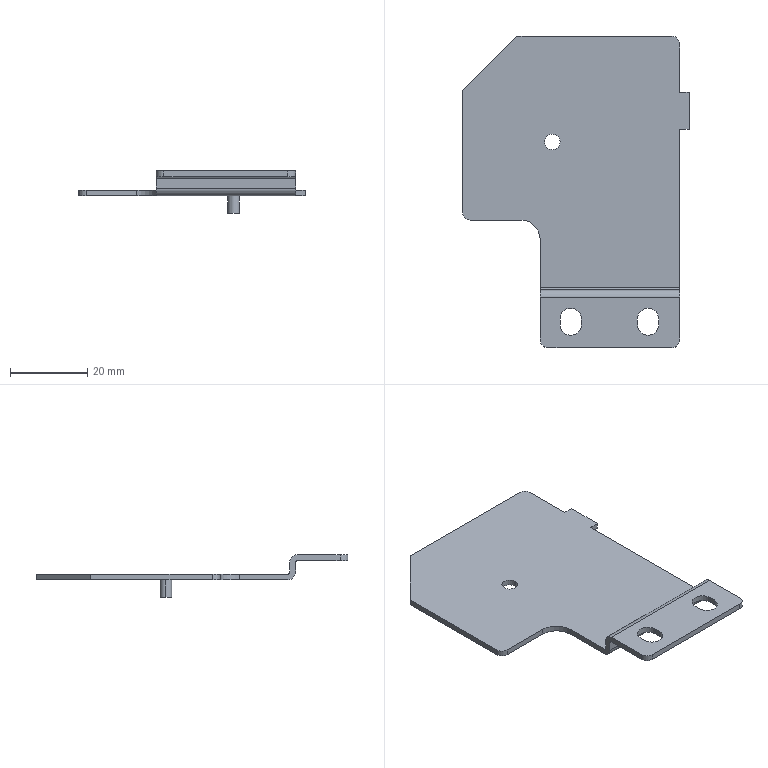Part | NX | features BREP 1 | 1 solid | 39 faces | box 58.5 x 80.5 x 11 mm | volume 5793 mm3 | plane 22 | cylinder 17 | commonest cylinder face diameters 4 x8 5.5 x4 1 x2 3 x2 10 x1
STEP:
#1=CARTESIAN_POINT('',(-6.875,12.95,1.));
#2=VERTEX_POINT('',#1);
#3=CARTESIAN_POINT('',(-2.875,12.95,1.));
#4=VERTEX_POINT('',#3);
#5=CARTESIAN_POINT('',(-4.875,12.95,1.));
#6=DIRECTION('',(0.,0.,1.));
#7=DIRECTION('',(1.,0.,0.));
#8=AXIS2_PLACEMENT_3D('',#5,#6,#7);
#9=CIRCLE('',#8,2.);
#10=EDGE_CURVE('',#2,#4,#9,.T.);
#11=ORIENTED_EDGE('',*,*,#10,.F.);
#12=CARTESIAN_POINT('',(-6.875,12.95,2.5));
#13=VERTEX_POINT('',#12);
#14=CARTESIAN_POINT('',(-6.875,12.95,1.));
#15=DIRECTION('',(0.,0.,1.));
#16=VECTOR('',#15,1000.);
#17=LINE('',#14,#16);
#18=EDGE_CURVE('',#2,#13,#17,.T.);
#19=ORIENTED_EDGE('',*,*,#18,.T.);
#20=CARTESIAN_POINT('',(-2.875,12.95,2.5));
#21=VERTEX_POINT('',#20);
#22=CARTESIAN_POINT('',(-4.875,12.95,2.5));
#23=DIRECTION('',(0.,0.,-1.));
#24=DIRECTION('',(1.,0.,0.));
#25=AXIS2_PLACEMENT_3D('',#22,#23,#24);
#26=CIRCLE('',#25,2.);
#27=EDGE_CURVE('',#21,#13,#26,.T.);
#28=ORIENTED_EDGE('',*,*,#27,.F.);
#29=CARTESIAN_POINT('',(-2.875,12.95,1.));
#30=DIRECTION('',(0.,0.,1.));
#31=VECTOR('',#30,1000.);
#32=LINE('',#29,#31);
#33=EDGE_CURVE('',#4,#21,#32,.T.);
#34=ORIENTED_EDGE('',*,*,#33,.F.);
#35=EDGE_LOOP('',(#11,#19,#28,#34));
#36=FACE_BOUND('',#35,.T.);
#37=CARTESIAN_POINT('',(-4.875,12.95,1.));
#38=DIRECTION('',(0.,0.,1.));
#39=DIRECTION('',(-1.,0.,0.));
#40=AXIS2_PLACEMENT_3D('',#37,#38,#39);
#41=CYLINDRICAL_SURFACE('',#40,2.);
#42=ADVANCED_FACE('',(#36),#41,.F.);
#43=CARTESIAN_POINT('',(10.5,6.75,1.));
#44=VERTEX_POINT('',#43);
#45=CARTESIAN_POINT('',(13.5,6.75,1.));
#46=VERTEX_POINT('',#45);
#47=CARTESIAN_POINT('',(12.,6.75,1.));
#48=DIRECTION('',(0.,0.,-1.));
#49=DIRECTION('',(-1.,0.,0.));
#50=AXIS2_PLACEMENT_3D('',#47,#48,#49);
#51=CIRCLE('',#50,1.5);
#52=EDGE_CURVE('',#44,#46,#51,.T.);
#53=ORIENTED_EDGE('',*,*,#52,.T.);
#54=CARTESIAN_POINT('',(13.5,6.75,-3.5));
#55=VERTEX_POINT('',#54);
#56=CARTESIAN_POINT('',(13.5,6.75,2.5));
#57=DIRECTION('',(0.,0.,-1.));
#58=VECTOR('',#57,1000.);
#59=LINE('',#56,#58);
#60=EDGE_CURVE('',#55,#46,#59,.F.);
#61=ORIENTED_EDGE('',*,*,#60,.F.);
#62=CARTESIAN_POINT('',(10.5,6.75,-3.5));
#63=VERTEX_POINT('',#62);
#64=CARTESIAN_POINT('',(12.,6.75,-3.5));
#65=DIRECTION('',(0.,0.,1.));
#66=DIRECTION('',(-1.,0.,0.));
#67=AXIS2_PLACEMENT_3D('',#64,#65,#66);
#68=CIRCLE('',#67,1.5);
#69=EDGE_CURVE('',#55,#63,#68,.T.);
#70=ORIENTED_EDGE('',*,*,#69,.T.);
#71=CARTESIAN_POINT('',(10.5,6.75,2.5));
#72=DIRECTION('',(0.,0.,-1.));
#73=VECTOR('',#72,1000.);
#74=LINE('',#71,#73);
#75=EDGE_CURVE('',#63,#44,#74,.F.);
#76=ORIENTED_EDGE('',*,*,#75,.T.);
#77=EDGE_LOOP('',(#53,#61,#70,#76));
#78=FACE_BOUND('',#77,.T.);
#79=CARTESIAN_POINT('',(12.,6.75,2.5));
#80=DIRECTION('',(0.,0.,-1.));
#81=DIRECTION('',(1.,0.,0.));
#82=AXIS2_PLACEMENT_3D('',#79,#80,#81);
#83=CYLINDRICAL_SURFACE('',#82,1.5);
#84=ADVANCED_FACE('',(#78),#83,.T.);
#85=CARTESIAN_POINT('',(-14.,40.25,2.5));
#86=VERTEX_POINT('',#85);
#87=CARTESIAN_POINT('',(-28.,26.25,2.5));
#88=VERTEX_POINT('',#87);
#89=CARTESIAN_POINT('',(-14.,40.25,2.5));
#90=DIRECTION('',(-0.7071,-0.7071,0.));
#91=VECTOR('',#90,1000.);
#92=LINE('',#89,#91);
#93=EDGE_CURVE('',#86,#88,#92,.T.);
#94=ORIENTED_EDGE('',*,*,#93,.T.);
#95=CARTESIAN_POINT('',(-28.,-5.25,2.5));
#96=VERTEX_POINT('',#95);
#97=CARTESIAN_POINT('',(-28.,-7.834,2.5));
#98=DIRECTION('',(0.,-1.,0.));
#99=VECTOR('',#98,1000.);
#100=LINE('',#97,#99);
#101=EDGE_CURVE('',#88,#96,#100,.T.);
#102=ORIENTED_EDGE('',*,*,#101,.T.);
#103=CARTESIAN_POINT('',(-26.,-7.25,2.5));
#104=VERTEX_POINT('',#103);
#105=CARTESIAN_POINT('',(-26.,-5.25,2.5));
#106=DIRECTION('',(0.,0.,1.));
#107=DIRECTION('',(1.,0.,0.));
#108=AXIS2_PLACEMENT_3D('',#105,#106,#107);
#109=CIRCLE('',#108,2.);
#110=EDGE_CURVE('',#96,#104,#109,.T.);
#111=ORIENTED_EDGE('',*,*,#110,.T.);
#112=CARTESIAN_POINT('',(-13.,-7.25,2.5));
#113=VERTEX_POINT('',#112);
#114=CARTESIAN_POINT('',(38.,-7.25,2.5));
#115=DIRECTION('',(1.,0.,0.));
#116=VECTOR('',#115,1000.);
#117=LINE('',#114,#116);
#118=EDGE_CURVE('',#104,#113,#117,.T.);
#119=ORIENTED_EDGE('',*,*,#118,.T.);
#120=CARTESIAN_POINT('',(-8.,-12.25,2.5));
#121=VERTEX_POINT('',#120);
#122=CARTESIAN_POINT('',(-13.,-12.25,2.5));
#123=DIRECTION('',(0.,0.,-1.));
#124=DIRECTION('',(1.,0.,0.));
#125=AXIS2_PLACEMENT_3D('',#122,#123,#124);
#126=CIRCLE('',#125,5.);
#127=EDGE_CURVE('',#113,#121,#126,.T.);
#128=ORIENTED_EDGE('',*,*,#127,.T.);
#129=CARTESIAN_POINT('',(-8.,-24.768,2.5));
#130=VERTEX_POINT('',#129);
#131=CARTESIAN_POINT('',(-8.,-7.834,2.5));
#132=DIRECTION('',(0.,-1.,0.));
#133=VECTOR('',#132,1000.);
#134=LINE('',#131,#133);
#135=EDGE_CURVE('',#121,#130,#134,.T.);
#136=ORIENTED_EDGE('',*,*,#135,.T.);
#137=CARTESIAN_POINT('',(28.,-24.768,2.5));
#138=VERTEX_POINT('',#137);
#139=CARTESIAN_POINT('',(38.,-24.768,2.5));
#140=DIRECTION('',(1.,0.,0.));
#141=VECTOR('',#140,1000.);
#142=LINE('',#139,#141);
#143=EDGE_CURVE('',#130,#138,#142,.T.);
#144=ORIENTED_EDGE('',*,*,#143,.T.);
#145=CARTESIAN_POINT('',(28.,16.25,2.5));
#146=VERTEX_POINT('',#145);
#147=CARTESIAN_POINT('',(28.,-7.834,2.5));
#148=DIRECTION('',(0.,1.,0.));
#149=VECTOR('',#148,1000.);
#150=LINE('',#147,#149);
#151=EDGE_CURVE('',#138,#146,#150,.T.);
#152=ORIENTED_EDGE('',*,*,#151,.T.);
#153=CARTESIAN_POINT('',(30.5,16.25,2.5));
#154=VERTEX_POINT('',#153);
#155=CARTESIAN_POINT('',(38.,16.25,2.5));
#156=DIRECTION('',(1.,0.,0.));
#157=VECTOR('',#156,1000.);
#158=LINE('',#155,#157);
#159=EDGE_CURVE('',#146,#154,#158,.T.);
#160=ORIENTED_EDGE('',*,*,#159,.T.);
#161=CARTESIAN_POINT('',(30.5,25.75,2.5));
#162=VERTEX_POINT('',#161);
#163=CARTESIAN_POINT('',(30.5,-7.834,2.5));
#164=DIRECTION('',(0.,1.,0.));
#165=VECTOR('',#164,1000.);
#166=LINE('',#163,#165);
#167=EDGE_CURVE('',#154,#162,#166,.T.);
#168=ORIENTED_EDGE('',*,*,#167,.T.);
#169=CARTESIAN_POINT('',(28.,25.75,2.5));
#170=VERTEX_POINT('',#169);
#171=CARTESIAN_POINT('',(38.,25.75,2.5));
#172=DIRECTION('',(-1.,0.,0.));
#173=VECTOR('',#172,1000.);
#174=LINE('',#171,#173);
#175=EDGE_CURVE('',#162,#170,#174,.T.);
#176=ORIENTED_EDGE('',*,*,#175,.T.);
#177=CARTESIAN_POINT('',(28.,38.25,2.5));
#178=VERTEX_POINT('',#177);
#179=CARTESIAN_POINT('',(28.,-7.834,2.5));
#180=DIRECTION('',(0.,1.,0.));
#181=VECTOR('',#180,1000.);
#182=LINE('',#179,#181);
#183=EDGE_CURVE('',#170,#178,#182,.T.);
#184=ORIENTED_EDGE('',*,*,#183,.T.);
#185=CARTESIAN_POINT('',(26.,40.25,2.5));
#186=VERTEX_POINT('',#185);
#187=CARTESIAN_POINT('',(26.,38.25,2.5));
#188=DIRECTION('',(0.,0.,1.));
#189=DIRECTION('',(1.,0.,0.));
#190=AXIS2_PLACEMENT_3D('',#187,#188,#189);
#191=CIRCLE('',#190,2.);
#192=EDGE_CURVE('',#178,#186,#191,.T.);
#193=ORIENTED_EDGE('',*,*,#192,.T.);
#194=CARTESIAN_POINT('',(38.,40.25,2.5));
#195=DIRECTION('',(-1.,0.,0.));
#196=VECTOR('',#195,1000.);
#197=LINE('',#194,#196);
#198=EDGE_CURVE('',#186,#86,#197,.T.);
#199=ORIENTED_EDGE('',*,*,#198,.T.);
#200=EDGE_LOOP('',(#94,#102,#111,#119,#128,#136,#144,#152,#160,#168,#176,#184,#193,#199));
#201=FACE_BOUND('',#200,.T.);
#202=ORIENTED_EDGE('',*,*,#27,.T.);
#203=CARTESIAN_POINT('',(-4.875,12.95,2.5));
#204=DIRECTION('',(0.,0.,-1.));
#205=DIRECTION('',(1.,0.,0.));
#206=AXIS2_PLACEMENT_3D('',#203,#204,#205);
#207=CIRCLE('',#206,2.);
#208=EDGE_CURVE('',#13,#21,#207,.T.);
#209=ORIENTED_EDGE('',*,*,#208,.T.);
#210=EDGE_LOOP('',(#202,#209));
#211=FACE_BOUND('',#210,.T.);
#212=CARTESIAN_POINT('',(38.,-7.834,2.5));
#213=DIRECTION('',(0.,0.,1.));
#214=DIRECTION('',(-1.,0.,0.));
#215=AXIS2_PLACEMENT_3D('',#212,#213,#214);
#216=PLANE('',#215);
#217=ADVANCED_FACE('',(#201,#211),#216,.T.);
#218=ORIENTED_EDGE('',*,*,#101,.F.);
#219=CARTESIAN_POINT('',(-28.,26.25,1.));
#220=VERTEX_POINT('',#219);
#221=CARTESIAN_POINT('',(-28.,26.25,1.));
#222=DIRECTION('',(0.,0.,-1.));
#223=VECTOR('',#222,1000.);
#224=LINE('',#221,#223);
#225=EDGE_CURVE('',#88,#220,#224,.T.);
#226=ORIENTED_EDGE('',*,*,#225,.T.);
#227=CARTESIAN_POINT('',(-28.,-5.25,1.));
#228=VERTEX_POINT('',#227);
#229=CARTESIAN_POINT('',(-28.,-7.834,1.));
#230=DIRECTION('',(0.,-1.,0.));
#231=VECTOR('',#230,1000.);
#232=LINE('',#229,#231);
#233=EDGE_CURVE('',#220,#228,#232,.T.);
#234=ORIENTED_EDGE('',*,*,#233,.T.);
#235=CARTESIAN_POINT('',(-28.,-5.25,1.));
#236=DIRECTION('',(0.,0.,1.));
#237=VECTOR('',#236,1000.);
#238=LINE('',#235,#237);
#239=EDGE_CURVE('',#228,#96,#238,.T.);
#240=ORIENTED_EDGE('',*,*,#239,.T.);
#241=EDGE_LOOP('',(#218,#226,#234,#240));
#242=FACE_BOUND('',#241,.T.);
#243=CARTESIAN_POINT('',(-28.,-7.834,1.));
#244=DIRECTION('',(-1.,0.,0.));
#245=DIRECTION('',(0.,0.,-1.));
#246=AXIS2_PLACEMENT_3D('',#243,#244,#245);
#247=PLANE('',#246);
#248=ADVANCED_FACE('',(#242),#247,.T.);
#249=CARTESIAN_POINT('',(-14.,40.25,1.));
#250=VERTEX_POINT('',#249);
#251=CARTESIAN_POINT('',(-14.,40.25,1.));
#252=DIRECTION('',(0.7071,0.7071,0.));
#253=VECTOR('',#252,1000.);
#254=LINE('',#251,#253);
#255=EDGE_CURVE('',#220,#250,#254,.T.);
#256=ORIENTED_EDGE('',*,*,#255,.F.);
#257=ORIENTED_EDGE('',*,*,#225,.F.);
#258=ORIENTED_EDGE('',*,*,#93,.F.);
#259=CARTESIAN_POINT('',(-14.,40.25,1.));
#260=DIRECTION('',(0.,0.,1.));
#261=VECTOR('',#260,1000.);
#262=LINE('',#259,#261);
#263=EDGE_CURVE('',#250,#86,#262,.T.);
#264=ORIENTED_EDGE('',*,*,#263,.F.);
#265=EDGE_LOOP('',(#256,#257,#258,#264));
#266=FACE_BOUND('',#265,.T.);
#267=CARTESIAN_POINT('',(-14.,40.25,1.));
#268=DIRECTION('',(0.7071,-0.7071,0.));
#269=DIRECTION('',(-0.7071,-0.7071,0.));
#270=AXIS2_PLACEMENT_3D('',#267,#268,#269);
#271=PLANE('',#270);
#272=ADVANCED_FACE('',(#266),#271,.F.);
#273=ORIENTED_EDGE('',*,*,#198,.F.);
#274=CARTESIAN_POINT('',(26.,40.25,1.));
#275=VERTEX_POINT('',#274);
#276=CARTESIAN_POINT('',(26.,40.25,1.));
#277=DIRECTION('',(0.,0.,-1.));
#278=VECTOR('',#277,1000.);
#279=LINE('',#276,#278);
#280=EDGE_CURVE('',#186,#275,#279,.T.);
#281=ORIENTED_EDGE('',*,*,#280,.T.);
#282=CARTESIAN_POINT('',(38.,40.25,1.));
#283=DIRECTION('',(-1.,0.,0.));
#284=VECTOR('',#283,1000.);
#285=LINE('',#282,#284);
#286=EDGE_CURVE('',#275,#250,#285,.T.);
#287=ORIENTED_EDGE('',*,*,#286,.T.);
#288=ORIENTED_EDGE('',*,*,#263,.T.);
#289=EDGE_LOOP('',(#273,#281,#287,#288));
#290=FACE_BOUND('',#289,.T.);
#291=CARTESIAN_POINT('',(38.,40.25,1.));
#292=DIRECTION('',(0.,1.,0.));
#293=DIRECTION('',(0.,0.,-1.));
#294=AXIS2_PLACEMENT_3D('',#291,#292,#293);
#295=PLANE('',#294);
#296=ADVANCED_FACE('',(#290),#295,.T.);
#297=ORIENTED_EDGE('',*,*,#192,.F.);
#298=CARTESIAN_POINT('',(28.,38.25,1.));
#299=VERTEX_POINT('',#298);
#300=CARTESIAN_POINT('',(28.,38.25,1.));
#301=DIRECTION('',(0.,0.,-1.));
#302=VECTOR('',#301,1000.);
#303=LINE('',#300,#302);
#304=EDGE_CURVE('',#178,#299,#303,.T.);
#305=ORIENTED_EDGE('',*,*,#304,.T.);
#306=CARTESIAN_POINT('',(26.,38.25,1.));
#307=DIRECTION('',(0.,0.,1.));
#308=DIRECTION('',(1.,0.,0.));
#309=AXIS2_PLACEMENT_3D('',#306,#307,#308);
#310=CIRCLE('',#309,2.);
#311=EDGE_CURVE('',#299,#275,#310,.T.);
#312=ORIENTED_EDGE('',*,*,#311,.T.);
#313=ORIENTED_EDGE('',*,*,#280,.F.);
#314=EDGE_LOOP('',(#297,#305,#312,#313));
#315=FACE_BOUND('',#314,.T.);
#316=CARTESIAN_POINT('',(26.,38.25,1.));
#317=DIRECTION('',(0.,0.,1.));
#318=DIRECTION('',(-1.,0.,0.));
#319=AXIS2_PLACEMENT_3D('',#316,#317,#318);
#320=CYLINDRICAL_SURFACE('',#319,2.);
#321=ADVANCED_FACE('',(#315),#320,.T.);
#322=ORIENTED_EDGE('',*,*,#183,.F.);
#323=CARTESIAN_POINT('',(28.,25.75,1.));
#324=VERTEX_POINT('',#323);
#325=CARTESIAN_POINT('',(28.,25.75,6.));
#326=DIRECTION('',(0.,0.,-1.));
#327=VECTOR('',#326,1000.);
#328=LINE('',#325,#327);
#329=EDGE_CURVE('',#170,#324,#328,.T.);
#330=ORIENTED_EDGE('',*,*,#329,.T.);
#331=CARTESIAN_POINT('',(28.,-36.323,1.));
#332=DIRECTION('',(0.,1.,0.));
#333=VECTOR('',#332,1000.);
#334=LINE('',#331,#333);
#335=EDGE_CURVE('',#324,#299,#334,.T.);
#336=ORIENTED_EDGE('',*,*,#335,.T.);
#337=ORIENTED_EDGE('',*,*,#304,.F.);
#338=EDGE_LOOP('',(#322,#330,#336,#337));
#339=FACE_BOUND('',#338,.T.);
#340=CARTESIAN_POINT('',(28.,-36.323,6.));
#341=DIRECTION('',(1.,0.,0.));
#342=DIRECTION('',(0.,0.,1.));
#343=AXIS2_PLACEMENT_3D('',#340,#341,#342);
#344=PLANE('',#343);
#345=ADVANCED_FACE('',(#339),#344,.T.);
#346=ORIENTED_EDGE('',*,*,#175,.F.);
#347=CARTESIAN_POINT('',(30.5,25.75,1.));
#348=VERTEX_POINT('',#347);
#349=CARTESIAN_POINT('',(30.5,25.75,1.));
#350=DIRECTION('',(0.,0.,-1.));
#351=VECTOR('',#350,1000.);
#352=LINE('',#349,#351);
#353=EDGE_CURVE('',#162,#348,#352,.T.);
#354=ORIENTED_EDGE('',*,*,#353,.T.);
#355=CARTESIAN_POINT('',(28.,25.75,1.));
#356=DIRECTION('',(-1.,0.,0.));
#357=VECTOR('',#356,1000.);
#358=LINE('',#355,#357);
#359=EDGE_CURVE('',#348,#324,#358,.T.);
#360=ORIENTED_EDGE('',*,*,#359,.T.);
#361=ORIENTED_EDGE('',*,*,#329,.F.);
#362=EDGE_LOOP('',(#346,#354,#360,#361));
#363=FACE_BOUND('',#362,.T.);
#364=CARTESIAN_POINT('',(28.,25.75,1.));
#365=DIRECTION('',(0.,1.,0.));
#366=DIRECTION('',(0.,0.,-1.));
#367=AXIS2_PLACEMENT_3D('',#364,#365,#366);
#368=PLANE('',#367);
#369=ADVANCED_FACE('',(#363),#368,.T.);
#370=ORIENTED_EDGE('',*,*,#167,.F.);
#371=CARTESIAN_POINT('',(30.5,16.25,1.));
#372=VERTEX_POINT('',#371);
#373=CARTESIAN_POINT('',(30.5,16.25,1.));
#374=DIRECTION('',(0.,0.,-1.));
#375=VECTOR('',#374,1000.);
#376=LINE('',#373,#375);
#377=EDGE_CURVE('',#154,#372,#376,.T.);
#378=ORIENTED_EDGE('',*,*,#377,.T.);
#379=CARTESIAN_POINT('',(30.5,16.25,1.));
#380=DIRECTION('',(0.,1.,0.));
#381=VECTOR('',#380,1000.);
#382=LINE('',#379,#381);
#383=EDGE_CURVE('',#372,#348,#382,.T.);
#384=ORIENTED_EDGE('',*,*,#383,.T.);
#385=ORIENTED_EDGE('',*,*,#353,.F.);
#386=EDGE_LOOP('',(#370,#378,#384,#385));
#387=FACE_BOUND('',#386,.T.);
#388=CARTESIAN_POINT('',(30.5,16.25,1.));
#389=DIRECTION('',(1.,0.,0.));
#390=DIRECTION('',(0.,0.,1.));
#391=AXIS2_PLACEMENT_3D('',#388,#389,#390);
#392=PLANE('',#391);
#393=ADVANCED_FACE('',(#387),#392,.T.);
#394=ORIENTED_EDGE('',*,*,#159,.F.);
#395=CARTESIAN_POINT('',(28.,16.25,1.));
#396=VERTEX_POINT('',#395);
#397=CARTESIAN_POINT('',(28.,16.25,1.));
#398=DIRECTION('',(0.,0.,-1.));
#399=VECTOR('',#398,1000.);
#400=LINE('',#397,#399);
#401=EDGE_CURVE('',#146,#396,#400,.T.);
#402=ORIENTED_EDGE('',*,*,#401,.T.);
#403=CARTESIAN_POINT('',(28.,16.25,1.));
#404=DIRECTION('',(1.,0.,0.));
#405=VECTOR('',#404,1000.);
#406=LINE('',#403,#405);
#407=EDGE_CURVE('',#396,#372,#406,.T.);
#408=ORIENTED_EDGE('',*,*,#407,.T.);
#409=ORIENTED_EDGE('',*,*,#377,.F.);
#410=EDGE_LOOP('',(#394,#402,#408,#409));
#411=FACE_BOUND('',#410,.T.);
#412=CARTESIAN_POINT('',(28.,16.25,1.));
#413=DIRECTION('',(0.,-1.,0.));
#414=DIRECTION('',(0.,0.,1.));
#415=AXIS2_PLACEMENT_3D('',#412,#413,#414);
#416=PLANE('',#415);
#417=ADVANCED_FACE('',(#411),#416,.T.);
#418=CARTESIAN_POINT('',(28.,-24.768,1.));
#419=VERTEX_POINT('',#418);
#420=CARTESIAN_POINT('',(28.,-36.323,1.));
#421=DIRECTION('',(0.,1.,0.));
#422=VECTOR('',#421,1000.);
#423=LINE('',#420,#422);
#424=EDGE_CURVE('',#419,#396,#423,.T.);
#425=ORIENTED_EDGE('',*,*,#424,.T.);
#426=ORIENTED_EDGE('',*,*,#401,.F.);
#427=ORIENTED_EDGE('',*,*,#151,.F.);
#428=CARTESIAN_POINT('',(28.,-25.268,3.));
#429=VERTEX_POINT('',#428);
#430=CARTESIAN_POINT('',(28.,-24.768,3.));
#431=DIRECTION('',(-1.,0.,0.));
#432=DIRECTION('',(0.,0.,-1.));
#433=AXIS2_PLACEMENT_3D('',#430,#431,#432);
#434=CIRCLE('',#433,0.5);
#435=EDGE_CURVE('',#138,#429,#434,.T.);
#436=ORIENTED_EDGE('',*,*,#435,.T.);
#437=CARTESIAN_POINT('',(28.,-25.268,5.5));
#438=VERTEX_POINT('',#437);
#439=CARTESIAN_POINT('',(28.,-25.268,6.));
#440=DIRECTION('',(0.,0.,1.));
#441=VECTOR('',#440,1000.);
#442=LINE('',#439,#441);
#443=EDGE_CURVE('',#429,#438,#442,.T.);
#444=ORIENTED_EDGE('',*,*,#443,.T.);
#445=CARTESIAN_POINT('',(28.,-27.268,7.5));
#446=VERTEX_POINT('',#445);
#447=CARTESIAN_POINT('',(28.,-27.268,5.5));
#448=DIRECTION('',(1.,0.,0.));
#449=DIRECTION('',(0.,0.,-1.));
#450=AXIS2_PLACEMENT_3D('',#447,#448,#449);
#451=CIRCLE('',#450,2.);
#452=EDGE_CURVE('',#438,#446,#451,.T.);
#453=ORIENTED_EDGE('',*,*,#452,.T.);
#454=CARTESIAN_POINT('',(28.,-38.25,7.5));
#455=VERTEX_POINT('',#454);
#456=CARTESIAN_POINT('',(28.,-36.323,7.5));
#457=DIRECTION('',(0.,-1.,0.));
#458=VECTOR('',#457,1000.);
#459=LINE('',#456,#458);
#460=EDGE_CURVE('',#446,#455,#459,.T.);
#461=ORIENTED_EDGE('',*,*,#460,.T.);
#462=CARTESIAN_POINT('',(28.,-38.25,6.));
#463=VERTEX_POINT('',#462);
#464=CARTESIAN_POINT('',(28.,-38.25,6.));
#465=DIRECTION('',(0.,0.,1.));
#466=VECTOR('',#465,1000.);
#467=LINE('',#464,#466);
#468=EDGE_CURVE('',#463,#455,#467,.T.);
#469=ORIENTED_EDGE('',*,*,#468,.F.);
#470=CARTESIAN_POINT('',(28.,-27.268,6.));
#471=VERTEX_POINT('',#470);
#472=CARTESIAN_POINT('',(28.,-36.323,6.));
#473=DIRECTION('',(0.,1.,0.));
#474=VECTOR('',#473,1000.);
#475=LINE('',#472,#474);
#476=EDGE_CURVE('',#463,#471,#475,.T.);
#477=ORIENTED_EDGE('',*,*,#476,.T.);
#478=CARTESIAN_POINT('',(28.,-26.768,5.5));
#479=VERTEX_POINT('',#478);
#480=CARTESIAN_POINT('',(28.,-27.268,5.5));
#481=DIRECTION('',(-1.,0.,0.));
#482=DIRECTION('',(0.,0.,-1.));
#483=AXIS2_PLACEMENT_3D('',#480,#481,#482);
#484=CIRCLE('',#483,0.5);
#485=EDGE_CURVE('',#471,#479,#484,.T.);
#486=ORIENTED_EDGE('',*,*,#485,.T.);
#487=CARTESIAN_POINT('',(28.,-26.768,3.));
#488=VERTEX_POINT('',#487);
#489=CARTESIAN_POINT('',(28.,-26.768,6.));
#490=DIRECTION('',(0.,0.,-1.));
#491=VECTOR('',#490,1000.);
#492=LINE('',#489,#491);
#493=EDGE_CURVE('',#479,#488,#492,.T.);
#494=ORIENTED_EDGE('',*,*,#493,.T.);
#495=CARTESIAN_POINT('',(28.,-24.768,3.));
#496=DIRECTION('',(1.,0.,0.));
#497=DIRECTION('',(0.,0.,-1.));
#498=AXIS2_PLACEMENT_3D('',#495,#496,#497);
#499=CIRCLE('',#498,2.);
#500=EDGE_CURVE('',#488,#419,#499,.T.);
#501=ORIENTED_EDGE('',*,*,#500,.T.);
#502=EDGE_LOOP('',(#425,#426,#427,#436,#444,#453,#461,#469,#477,#486,#494,#501));
#503=FACE_BOUND('',#502,.T.);
#504=CARTESIAN_POINT('',(28.,-36.323,6.));
#505=DIRECTION('',(1.,0.,0.));
#506=DIRECTION('',(0.,0.,1.));
#507=AXIS2_PLACEMENT_3D('',#504,#505,#506);
#508=PLANE('',#507);
#509=ADVANCED_FACE('',(#503),#508,.T.);
#510=ORIENTED_EDGE('',*,*,#435,.F.);
#511=ORIENTED_EDGE('',*,*,#143,.F.);
#512=CARTESIAN_POINT('',(-8.,-25.268,3.));
#513=VERTEX_POINT('',#512);
#514=CARTESIAN_POINT('',(-8.,-24.768,3.));
#515=DIRECTION('',(1.,0.,0.));
#516=DIRECTION('',(0.,0.,-1.));
#517=AXIS2_PLACEMENT_3D('',#514,#515,#516);
#518=CIRCLE('',#517,0.5);
#519=EDGE_CURVE('',#513,#130,#518,.T.);
#520=ORIENTED_EDGE('',*,*,#519,.F.);
#521=CARTESIAN_POINT('',(46.085,-25.268,3.));
#522=DIRECTION('',(-1.,0.,0.));
#523=VECTOR('',#522,1000.);
#524=LINE('',#521,#523);
#525=EDGE_CURVE('',#429,#513,#524,.T.);
#526=ORIENTED_EDGE('',*,*,#525,.F.);
#527=EDGE_LOOP('',(#510,#511,#520,#526));
#528=FACE_BOUND('',#527,.T.);
#529=CARTESIAN_POINT('',(46.085,-24.768,3.));
#530=DIRECTION('',(1.,0.,0.));
#531=DIRECTION('',(0.,0.,1.));
#532=AXIS2_PLACEMENT_3D('',#529,#530,#531);
#533=CYLINDRICAL_SURFACE('',#532,0.5);
#534=ADVANCED_FACE('',(#528),#533,.F.);
#535=ORIENTED_EDGE('',*,*,#135,.F.);
#536=CARTESIAN_POINT('',(-8.,-12.25,1.));
#537=VERTEX_POINT('',#536);
#538=CARTESIAN_POINT('',(-8.,-12.25,6.));
#539=DIRECTION('',(0.,0.,-1.));
#540=VECTOR('',#539,1000.);
#541=LINE('',#538,#540);
#542=EDGE_CURVE('',#121,#537,#541,.T.);
#543=ORIENTED_EDGE('',*,*,#542,.T.);
#544=CARTESIAN_POINT('',(-8.,-24.768,1.));
#545=VERTEX_POINT('',#544);
#546=CARTESIAN_POINT('',(-8.,32.708,1.));
#547=DIRECTION('',(0.,-1.,0.));
#548=VECTOR('',#547,1000.);
#549=LINE('',#546,#548);
#550=EDGE_CURVE('',#537,#545,#549,.T.);
#551=ORIENTED_EDGE('',*,*,#550,.T.);
#552=CARTESIAN_POINT('',(-8.,-26.768,3.));
#553=VERTEX_POINT('',#552);
#554=CARTESIAN_POINT('',(-8.,-24.768,3.));
#555=DIRECTION('',(-1.,0.,0.));
#556=DIRECTION('',(0.,0.,-1.));
#557=AXIS2_PLACEMENT_3D('',#554,#555,#556);
#558=CIRCLE('',#557,2.);
#559=EDGE_CURVE('',#545,#553,#558,.T.);
#560=ORIENTED_EDGE('',*,*,#559,.T.);
#561=CARTESIAN_POINT('',(-8.,-26.768,5.5));
#562=VERTEX_POINT('',#561);
#563=CARTESIAN_POINT('',(-8.,-26.768,6.));
#564=DIRECTION('',(0.,0.,1.));
#565=VECTOR('',#564,1000.);
#566=LINE('',#563,#565);
#567=EDGE_CURVE('',#553,#562,#566,.T.);
#568=ORIENTED_EDGE('',*,*,#567,.T.);
#569=CARTESIAN_POINT('',(-8.,-27.268,6.));
#570=VERTEX_POINT('',#569);
#571=CARTESIAN_POINT('',(-8.,-27.268,5.5));
#572=DIRECTION('',(1.,0.,0.));
#573=DIRECTION('',(0.,0.,-1.));
#574=AXIS2_PLACEMENT_3D('',#571,#572,#573);
#575=CIRCLE('',#574,0.5);
#576=EDGE_CURVE('',#562,#570,#575,.T.);
#577=ORIENTED_EDGE('',*,*,#576,.T.);
#578=CARTESIAN_POINT('',(-8.,-38.25,6.));
#579=VERTEX_POINT('',#578);
#580=CARTESIAN_POINT('',(-8.,32.708,6.));
#581=DIRECTION('',(0.,-1.,0.));
#582=VECTOR('',#581,1000.);
#583=LINE('',#580,#582);
#584=EDGE_CURVE('',#570,#579,#583,.T.);
#585=ORIENTED_EDGE('',*,*,#584,.T.);
#586=CARTESIAN_POINT('',(-8.,-38.25,7.5));
#587=VERTEX_POINT('',#586);
#588=CARTESIAN_POINT('',(-8.,-38.25,6.));
#589=DIRECTION('',(0.,0.,-1.));
#590=VECTOR('',#589,1000.);
#591=LINE('',#588,#590);
#592=EDGE_CURVE('',#587,#579,#591,.T.);
#593=ORIENTED_EDGE('',*,*,#592,.F.);
#594=CARTESIAN_POINT('',(-8.,-27.268,7.5));
#595=VERTEX_POINT('',#594);
#596=CARTESIAN_POINT('',(-8.,32.708,7.5));
#597=DIRECTION('',(0.,1.,0.));
#598=VECTOR('',#597,1000.);
#599=LINE('',#596,#598);
#600=EDGE_CURVE('',#587,#595,#599,.T.);
#601=ORIENTED_EDGE('',*,*,#600,.T.);
#602=CARTESIAN_POINT('',(-8.,-25.268,5.5));
#603=VERTEX_POINT('',#602);
#604=CARTESIAN_POINT('',(-8.,-27.268,5.5));
#605=DIRECTION('',(-1.,0.,0.));
#606=DIRECTION('',(0.,0.,-1.));
#607=AXIS2_PLACEMENT_3D('',#604,#605,#606);
#608=CIRCLE('',#607,2.);
#609=EDGE_CURVE('',#595,#603,#608,.T.);
#610=ORIENTED_EDGE('',*,*,#609,.T.);
#611=CARTESIAN_POINT('',(-8.,-25.268,6.));
#612=DIRECTION('',(0.,0.,-1.));
#613=VECTOR('',#612,1000.);
#614=LINE('',#611,#613);
#615=EDGE_CURVE('',#603,#513,#614,.T.);
#616=ORIENTED_EDGE('',*,*,#615,.T.);
#617=ORIENTED_EDGE('',*,*,#519,.T.);
#618=EDGE_LOOP('',(#535,#543,#551,#560,#568,#577,#585,#593,#601,#610,#616,#617));
#619=FACE_BOUND('',#618,.T.);
#620=CARTESIAN_POINT('',(-8.,32.708,6.));
#621=DIRECTION('',(-1.,0.,0.));
#622=DIRECTION('',(0.,0.,-1.));
#623=AXIS2_PLACEMENT_3D('',#620,#621,#622);
#624=PLANE('',#623);
#625=ADVANCED_FACE('',(#619),#624,.T.);
#626=ORIENTED_EDGE('',*,*,#542,.F.);
#627=ORIENTED_EDGE('',*,*,#127,.F.);
#628=CARTESIAN_POINT('',(-13.,-7.25,1.));
#629=VERTEX_POINT('',#628);
#630=CARTESIAN_POINT('',(-13.,-7.25,1.));
#631=DIRECTION('',(0.,0.,1.));
#632=VECTOR('',#631,1000.);
#633=LINE('',#630,#632);
#634=EDGE_CURVE('',#629,#113,#633,.T.);
#635=ORIENTED_EDGE('',*,*,#634,.F.);
#636=CARTESIAN_POINT('',(-13.,-12.25,1.));
#637=DIRECTION('',(0.,0.,1.));
#638=DIRECTION('',(1.,0.,0.));
#639=AXIS2_PLACEMENT_3D('',#636,#637,#638);
#640=CIRCLE('',#639,5.);
#641=EDGE_CURVE('',#537,#629,#640,.T.);
#642=ORIENTED_EDGE('',*,*,#641,.F.);
#643=EDGE_LOOP('',(#626,#627,#635,#642));
#644=FACE_BOUND('',#643,.T.);
#645=CARTESIAN_POINT('',(-13.,-12.25,1.));
#646=DIRECTION('',(0.,0.,1.));
#647=DIRECTION('',(-1.,0.,0.));
#648=AXIS2_PLACEMENT_3D('',#645,#646,#647);
#649=CYLINDRICAL_SURFACE('',#648,5.);
#650=ADVANCED_FACE('',(#644),#649,.F.);
#651=CARTESIAN_POINT('',(-26.,-7.25,1.));
#652=VERTEX_POINT('',#651);
#653=CARTESIAN_POINT('',(-26.,-7.25,1.));
#654=DIRECTION('',(0.,0.,1.));
#655=VECTOR('',#654,1000.);
#656=LINE('',#653,#655);
#657=EDGE_CURVE('',#652,#104,#656,.T.);
#658=ORIENTED_EDGE('',*,*,#657,.F.);
#659=CARTESIAN_POINT('',(38.,-7.25,1.));
#660=DIRECTION('',(-1.,0.,0.));
#661=VECTOR('',#660,1000.);
#662=LINE('',#659,#661);
#663=EDGE_CURVE('',#629,#652,#662,.T.);
#664=ORIENTED_EDGE('',*,*,#663,.F.);
#665=ORIENTED_EDGE('',*,*,#634,.T.);
#666=ORIENTED_EDGE('',*,*,#118,.F.);
#667=EDGE_LOOP('',(#658,#664,#665,#666));
#668=FACE_BOUND('',#667,.T.);
#669=CARTESIAN_POINT('',(38.,-7.25,1.));
#670=DIRECTION('',(0.,1.,0.));
#671=DIRECTION('',(0.,0.,-1.));
#672=AXIS2_PLACEMENT_3D('',#669,#670,#671);
#673=PLANE('',#672);
#674=ADVANCED_FACE('',(#668),#673,.F.);
#675=ORIENTED_EDGE('',*,*,#110,.F.);
#676=ORIENTED_EDGE('',*,*,#239,.F.);
#677=CARTESIAN_POINT('',(-26.,-5.25,1.));
#678=DIRECTION('',(0.,0.,1.));
#679=DIRECTION('',(1.,0.,0.));
#680=AXIS2_PLACEMENT_3D('',#677,#678,#679);
#681=CIRCLE('',#680,2.);
#682=EDGE_CURVE('',#228,#652,#681,.T.);
#683=ORIENTED_EDGE('',*,*,#682,.T.);
#684=ORIENTED_EDGE('',*,*,#657,.T.);
#685=EDGE_LOOP('',(#675,#676,#683,#684));
#686=FACE_BOUND('',#685,.T.);
#687=CARTESIAN_POINT('',(-26.,-5.25,1.));
#688=DIRECTION('',(0.,0.,1.));
#689=DIRECTION('',(-1.,0.,0.));
#690=AXIS2_PLACEMENT_3D('',#687,#688,#689);
#691=CYLINDRICAL_SURFACE('',#690,2.);
#692=ADVANCED_FACE('',(#686),#691,.T.);
#693=ORIENTED_EDGE('',*,*,#18,.F.);
#694=CARTESIAN_POINT('',(-4.875,12.95,1.));
#695=DIRECTION('',(0.,0.,1.));
#696=DIRECTION('',(1.,0.,0.));
#697=AXIS2_PLACEMENT_3D('',#694,#695,#696);
#698=CIRCLE('',#697,2.);
#699=EDGE_CURVE('',#4,#2,#698,.T.);
#700=ORIENTED_EDGE('',*,*,#699,.F.);
#701=ORIENTED_EDGE('',*,*,#33,.T.);
#702=ORIENTED_EDGE('',*,*,#208,.F.);
#703=EDGE_LOOP('',(#693,#700,#701,#702));
#704=FACE_BOUND('',#703,.T.);
#705=CARTESIAN_POINT('',(-4.875,12.95,1.));
#706=DIRECTION('',(0.,0.,1.));
#707=DIRECTION('',(-1.,0.,0.));
#708=AXIS2_PLACEMENT_3D('',#705,#706,#707);
#709=CYLINDRICAL_SURFACE('',#708,2.);
#710=ADVANCED_FACE('',(#704),#709,.F.);
#711=ORIENTED_EDGE('',*,*,#663,.T.);
#712=ORIENTED_EDGE('',*,*,#682,.F.);
#713=ORIENTED_EDGE('',*,*,#233,.F.);
#714=ORIENTED_EDGE('',*,*,#255,.T.);
#715=ORIENTED_EDGE('',*,*,#286,.F.);
#716=ORIENTED_EDGE('',*,*,#311,.F.);
#717=ORIENTED_EDGE('',*,*,#335,.F.);
#718=ORIENTED_EDGE('',*,*,#359,.F.);
#719=ORIENTED_EDGE('',*,*,#383,.F.);
#720=ORIENTED_EDGE('',*,*,#407,.F.);
#721=ORIENTED_EDGE('',*,*,#424,.F.);
#722=CARTESIAN_POINT('',(38.,-24.768,1.));
#723=DIRECTION('',(1.,0.,0.));
#724=VECTOR('',#723,1000.);
#725=LINE('',#722,#724);
#726=EDGE_CURVE('',#545,#419,#725,.T.);
#727=ORIENTED_EDGE('',*,*,#726,.F.);
#728=ORIENTED_EDGE('',*,*,#550,.F.);
#729=ORIENTED_EDGE('',*,*,#641,.T.);
#730=EDGE_LOOP('',(#711,#712,#713,#714,#715,#716,#717,#718,#719,#720,#721,#727,#728,#729));
#731=FACE_BOUND('',#730,.T.);
#732=ORIENTED_EDGE('',*,*,#699,.T.);
#733=ORIENTED_EDGE('',*,*,#10,.T.);
#734=EDGE_LOOP('',(#732,#733));
#735=FACE_BOUND('',#734,.T.);
#736=ORIENTED_EDGE('',*,*,#52,.F.);
#737=CARTESIAN_POINT('',(12.,6.75,1.));
#738=DIRECTION('',(0.,0.,-1.));
#739=DIRECTION('',(-1.,0.,0.));
#740=AXIS2_PLACEMENT_3D('',#737,#738,#739);
#741=CIRCLE('',#740,1.5);
#742=EDGE_CURVE('',#46,#44,#741,.T.);
#743=ORIENTED_EDGE('',*,*,#742,.F.);
#744=EDGE_LOOP('',(#736,#743));
#745=FACE_BOUND('',#744,.T.);
#746=CARTESIAN_POINT('',(38.,-7.834,1.));
#747=DIRECTION('',(0.,0.,1.));
#748=DIRECTION('',(-1.,0.,0.));
#749=AXIS2_PLACEMENT_3D('',#746,#747,#748);
#750=PLANE('',#749);
#751=ADVANCED_FACE('',(#731,#735,#745),#750,.F.);
#752=ORIENTED_EDGE('',*,*,#500,.F.);
#753=CARTESIAN_POINT('',(46.085,-26.768,3.));
#754=DIRECTION('',(-1.,0.,0.));
#755=VECTOR('',#754,1000.);
#756=LINE('',#753,#755);
#757=EDGE_CURVE('',#488,#553,#756,.T.);
#758=ORIENTED_EDGE('',*,*,#757,.T.);
#759=ORIENTED_EDGE('',*,*,#559,.F.);
#760=ORIENTED_EDGE('',*,*,#726,.T.);
#761=EDGE_LOOP('',(#752,#758,#759,#760));
#762=FACE_BOUND('',#761,.T.);
#763=CARTESIAN_POINT('',(46.085,-24.768,3.));
#764=DIRECTION('',(1.,0.,0.));
#765=DIRECTION('',(0.,0.,1.));
#766=AXIS2_PLACEMENT_3D('',#763,#764,#765);
#767=CYLINDRICAL_SURFACE('',#766,2.);
#768=ADVANCED_FACE('',(#762),#767,.T.);
#769=ORIENTED_EDGE('',*,*,#493,.F.);
#770=CARTESIAN_POINT('',(38.,-26.768,5.5));
#771=DIRECTION('',(1.,0.,0.));
#772=VECTOR('',#771,1000.);
#773=LINE('',#770,#772);
#774=EDGE_CURVE('',#562,#479,#773,.T.);
#775=ORIENTED_EDGE('',*,*,#774,.F.);
#776=ORIENTED_EDGE('',*,*,#567,.F.);
#777=ORIENTED_EDGE('',*,*,#757,.F.);
#778=EDGE_LOOP('',(#769,#775,#776,#777));
#779=FACE_BOUND('',#778,.T.);
#780=CARTESIAN_POINT('',(38.,-26.768,-15.898));
#781=DIRECTION('',(0.,1.,0.));
#782=DIRECTION('',(0.,0.,-1.));
#783=AXIS2_PLACEMENT_3D('',#780,#781,#782);
#784=PLANE('',#783);
#785=ADVANCED_FACE('',(#779),#784,.F.);
#786=CARTESIAN_POINT('',(26.,-40.25,6.));
#787=VERTEX_POINT('',#786);
#788=CARTESIAN_POINT('',(26.,-38.25,6.));
#789=DIRECTION('',(0.,0.,1.));
#790=DIRECTION('',(1.,0.,0.));
#791=AXIS2_PLACEMENT_3D('',#788,#789,#790);
#792=CIRCLE('',#791,2.);
#793=EDGE_CURVE('',#787,#463,#792,.T.);
#794=ORIENTED_EDGE('',*,*,#793,.F.);
#795=CARTESIAN_POINT('',(-6.,-40.25,6.));
#796=VERTEX_POINT('',#795);
#797=CARTESIAN_POINT('',(38.,-40.25,6.));
#798=DIRECTION('',(1.,0.,0.));
#799=VECTOR('',#798,1000.);
#800=LINE('',#797,#799);
#801=EDGE_CURVE('',#796,#787,#800,.T.);
#802=ORIENTED_EDGE('',*,*,#801,.F.);
#803=CARTESIAN_POINT('',(-6.,-38.25,6.));
#804=DIRECTION('',(0.,0.,1.));
#805=DIRECTION('',(1.,0.,0.));
#806=AXIS2_PLACEMENT_3D('',#803,#804,#805);
#807=CIRCLE('',#806,2.);
#808=EDGE_CURVE('',#579,#796,#807,.T.);
#809=ORIENTED_EDGE('',*,*,#808,.F.);
#810=ORIENTED_EDGE('',*,*,#584,.F.);
#811=CARTESIAN_POINT('',(38.,-27.268,6.));
#812=DIRECTION('',(-1.,0.,0.));
#813=VECTOR('',#812,1000.);
#814=LINE('',#811,#813);
#815=EDGE_CURVE('',#471,#570,#814,.T.);
#816=ORIENTED_EDGE('',*,*,#815,.F.);
#817=ORIENTED_EDGE('',*,*,#476,.F.);
#818=EDGE_LOOP('',(#794,#802,#809,#810,#816,#817));
#819=FACE_BOUND('',#818,.T.);
#820=CARTESIAN_POINT('',(22.625,-32.8,6.));
#821=VERTEX_POINT('',#820);
#822=CARTESIAN_POINT('',(22.625,-34.3,6.));
#823=VERTEX_POINT('',#822);
#824=CARTESIAN_POINT('',(22.625,-3.907,6.));
#825=DIRECTION('',(0.,-1.,0.));
#826=VECTOR('',#825,1000.);
#827=LINE('',#824,#826);
#828=EDGE_CURVE('',#821,#823,#827,.T.);
#829=ORIENTED_EDGE('',*,*,#828,.F.);
#830=CARTESIAN_POINT('',(17.125,-32.8,6.));
#831=VERTEX_POINT('',#830);
#832=CARTESIAN_POINT('',(19.875,-32.8,6.));
#833=DIRECTION('',(0.,0.,-1.));
#834=DIRECTION('',(1.,0.,0.));
#835=AXIS2_PLACEMENT_3D('',#832,#833,#834);
#836=CIRCLE('',#835,2.75);
#837=EDGE_CURVE('',#831,#821,#836,.T.);
#838=ORIENTED_EDGE('',*,*,#837,.F.);
#839=CARTESIAN_POINT('',(17.125,-34.3,6.));
#840=VERTEX_POINT('',#839);
#841=CARTESIAN_POINT('',(17.125,-3.907,6.));
#842=DIRECTION('',(0.,1.,0.));
#843=VECTOR('',#842,1000.);
#844=LINE('',#841,#843);
#845=EDGE_CURVE('',#840,#831,#844,.T.);
#846=ORIENTED_EDGE('',*,*,#845,.F.);
#847=CARTESIAN_POINT('',(19.875,-34.3,6.));
#848=DIRECTION('',(0.,0.,-1.));
#849=DIRECTION('',(1.,0.,0.));
#850=AXIS2_PLACEMENT_3D('',#847,#848,#849);
#851=CIRCLE('',#850,2.75);
#852=EDGE_CURVE('',#823,#840,#851,.T.);
#853=ORIENTED_EDGE('',*,*,#852,.F.);
#854=EDGE_LOOP('',(#829,#838,#846,#853));
#855=FACE_BOUND('',#854,.T.);
#856=CARTESIAN_POINT('',(2.625,-32.8,6.));
#857=VERTEX_POINT('',#856);
#858=CARTESIAN_POINT('',(2.625,-34.3,6.));
#859=VERTEX_POINT('',#858);
#860=CARTESIAN_POINT('',(2.625,-3.907,6.));
#861=DIRECTION('',(0.,-1.,0.));
#862=VECTOR('',#861,1000.);
#863=LINE('',#860,#862);
#864=EDGE_CURVE('',#857,#859,#863,.T.);
#865=ORIENTED_EDGE('',*,*,#864,.F.);
#866=CARTESIAN_POINT('',(-2.875,-32.8,6.));
#867=VERTEX_POINT('',#866);
#868=CARTESIAN_POINT('',(-0.125,-32.8,6.));
#869=DIRECTION('',(0.,0.,-1.));
#870=DIRECTION('',(1.,0.,0.));
#871=AXIS2_PLACEMENT_3D('',#868,#869,#870);
#872=CIRCLE('',#871,2.75);
#873=EDGE_CURVE('',#867,#857,#872,.T.);
#874=ORIENTED_EDGE('',*,*,#873,.F.);
#875=CARTESIAN_POINT('',(-2.875,-34.3,6.));
#876=VERTEX_POINT('',#875);
#877=CARTESIAN_POINT('',(-2.875,-3.907,6.));
#878=DIRECTION('',(0.,1.,0.));
#879=VECTOR('',#878,1000.);
#880=LINE('',#877,#879);
#881=EDGE_CURVE('',#876,#867,#880,.T.);
#882=ORIENTED_EDGE('',*,*,#881,.F.);
#883=CARTESIAN_POINT('',(-0.125,-34.3,6.));
#884=DIRECTION('',(0.,0.,-1.));
#885=DIRECTION('',(1.,0.,0.));
#886=AXIS2_PLACEMENT_3D('',#883,#884,#885);
#887=CIRCLE('',#886,2.75);
#888=EDGE_CURVE('',#859,#876,#887,.T.);
#889=ORIENTED_EDGE('',*,*,#888,.F.);
#890=EDGE_LOOP('',(#865,#874,#882,#889));
#891=FACE_BOUND('',#890,.T.);
#892=CARTESIAN_POINT('',(38.,-3.907,6.));
#893=DIRECTION('',(0.,0.,1.));
#894=DIRECTION('',(-1.,0.,0.));
#895=AXIS2_PLACEMENT_3D('',#892,#893,#894);
#896=PLANE('',#895);
#897=ADVANCED_FACE('',(#819,#855,#891),#896,.F.);
#898=CARTESIAN_POINT('',(-6.,-40.25,7.5));
#899=VERTEX_POINT('',#898);
#900=CARTESIAN_POINT('',(26.,-40.25,7.5));
#901=VERTEX_POINT('',#900);
#902=CARTESIAN_POINT('',(38.,-40.25,7.5));
#903=DIRECTION('',(1.,0.,0.));
#904=VECTOR('',#903,1000.);
#905=LINE('',#902,#904);
#906=EDGE_CURVE('',#899,#901,#905,.T.);
#907=ORIENTED_EDGE('',*,*,#906,.T.);
#908=CARTESIAN_POINT('',(26.,-38.25,7.5));
#909=DIRECTION('',(0.,0.,1.));
#910=DIRECTION('',(1.,0.,0.));
#911=AXIS2_PLACEMENT_3D('',#908,#909,#910);
#912=CIRCLE('',#911,2.);
#913=EDGE_CURVE('',#901,#455,#912,.T.);
#914=ORIENTED_EDGE('',*,*,#913,.T.);
#915=ORIENTED_EDGE('',*,*,#460,.F.);
#916=CARTESIAN_POINT('',(38.,-27.268,7.5));
#917=DIRECTION('',(-1.,0.,0.));
#918=VECTOR('',#917,1000.);
#919=LINE('',#916,#918);
#920=EDGE_CURVE('',#446,#595,#919,.T.);
#921=ORIENTED_EDGE('',*,*,#920,.T.);
#922=ORIENTED_EDGE('',*,*,#600,.F.);
#923=CARTESIAN_POINT('',(-6.,-38.25,7.5));
#924=DIRECTION('',(0.,0.,1.));
#925=DIRECTION('',(1.,0.,0.));
#926=AXIS2_PLACEMENT_3D('',#923,#924,#925);
#927=CIRCLE('',#926,2.);
#928=EDGE_CURVE('',#587,#899,#927,.T.);
#929=ORIENTED_EDGE('',*,*,#928,.T.);
#930=EDGE_LOOP('',(#907,#914,#915,#921,#922,#929));
#931=FACE_BOUND('',#930,.T.);
#932=CARTESIAN_POINT('',(2.625,-32.8,7.5));
#933=VERTEX_POINT('',#932);
#934=CARTESIAN_POINT('',(2.625,-34.3,7.5));
#935=VERTEX_POINT('',#934);
#936=CARTESIAN_POINT('',(2.625,-3.907,7.5));
#937=DIRECTION('',(0.,-1.,0.));
#938=VECTOR('',#937,1000.);
#939=LINE('',#936,#938);
#940=EDGE_CURVE('',#933,#935,#939,.T.);
#941=ORIENTED_EDGE('',*,*,#940,.T.);
#942=CARTESIAN_POINT('',(-2.875,-34.3,7.5));
#943=VERTEX_POINT('',#942);
#944=CARTESIAN_POINT('',(-0.125,-34.3,7.5));
#945=DIRECTION('',(0.,0.,-1.));
#946=DIRECTION('',(1.,0.,0.));
#947=AXIS2_PLACEMENT_3D('',#944,#945,#946);
#948=CIRCLE('',#947,2.75);
#949=EDGE_CURVE('',#935,#943,#948,.T.);
#950=ORIENTED_EDGE('',*,*,#949,.T.);
#951=CARTESIAN_POINT('',(-2.875,-32.8,7.5));
#952=VERTEX_POINT('',#951);
#953=CARTESIAN_POINT('',(-2.875,-3.907,7.5));
#954=DIRECTION('',(0.,1.,0.));
#955=VECTOR('',#954,1000.);
#956=LINE('',#953,#955);
#957=EDGE_CURVE('',#943,#952,#956,.T.);
#958=ORIENTED_EDGE('',*,*,#957,.T.);
#959=CARTESIAN_POINT('',(-0.125,-32.8,7.5));
#960=DIRECTION('',(0.,0.,-1.));
#961=DIRECTION('',(1.,0.,0.));
#962=AXIS2_PLACEMENT_3D('',#959,#960,#961);
#963=CIRCLE('',#962,2.75);
#964=EDGE_CURVE('',#952,#933,#963,.T.);
#965=ORIENTED_EDGE('',*,*,#964,.T.);
#966=EDGE_LOOP('',(#941,#950,#958,#965));
#967=FACE_BOUND('',#966,.T.);
#968=CARTESIAN_POINT('',(22.625,-32.8,7.5));
#969=VERTEX_POINT('',#968);
#970=CARTESIAN_POINT('',(22.625,-34.3,7.5));
#971=VERTEX_POINT('',#970);
#972=CARTESIAN_POINT('',(22.625,-3.907,7.5));
#973=DIRECTION('',(0.,-1.,0.));
#974=VECTOR('',#973,1000.);
#975=LINE('',#972,#974);
#976=EDGE_CURVE('',#969,#971,#975,.T.);
#977=ORIENTED_EDGE('',*,*,#976,.T.);
#978=CARTESIAN_POINT('',(17.125,-34.3,7.5));
#979=VERTEX_POINT('',#978);
#980=CARTESIAN_POINT('',(19.875,-34.3,7.5));
#981=DIRECTION('',(0.,0.,-1.));
#982=DIRECTION('',(1.,0.,0.));
#983=AXIS2_PLACEMENT_3D('',#980,#981,#982);
#984=CIRCLE('',#983,2.75);
#985=EDGE_CURVE('',#971,#979,#984,.T.);
#986=ORIENTED_EDGE('',*,*,#985,.T.);
#987=CARTESIAN_POINT('',(17.125,-32.8,7.5));
#988=VERTEX_POINT('',#987);
#989=CARTESIAN_POINT('',(17.125,-3.907,7.5));
#990=DIRECTION('',(0.,1.,0.));
#991=VECTOR('',#990,1000.);
#992=LINE('',#989,#991);
#993=EDGE_CURVE('',#979,#988,#992,.T.);
#994=ORIENTED_EDGE('',*,*,#993,.T.);
#995=CARTESIAN_POINT('',(19.875,-32.8,7.5));
#996=DIRECTION('',(0.,0.,-1.));
#997=DIRECTION('',(1.,0.,0.));
#998=AXIS2_PLACEMENT_3D('',#995,#996,#997);
#999=CIRCLE('',#998,2.75);
#1000=EDGE_CURVE('',#988,#969,#999,.T.);
#1001=ORIENTED_EDGE('',*,*,#1000,.T.);
#1002=EDGE_LOOP('',(#977,#986,#994,#1001));
#1003=FACE_BOUND('',#1002,.T.);
#1004=CARTESIAN_POINT('',(38.,-3.907,7.5));
#1005=DIRECTION('',(0.,0.,1.));
#1006=DIRECTION('',(-1.,0.,0.));
#1007=AXIS2_PLACEMENT_3D('',#1004,#1005,#1006);
#1008=PLANE('',#1007);
#1009=ADVANCED_FACE('',(#931,#967,#1003),#1008,.T.);
#1010=ORIENTED_EDGE('',*,*,#609,.F.);
#1011=ORIENTED_EDGE('',*,*,#920,.F.);
#1012=ORIENTED_EDGE('',*,*,#452,.F.);
#1013=CARTESIAN_POINT('',(46.085,-25.268,5.5));
#1014=DIRECTION('',(-1.,0.,0.));
#1015=VECTOR('',#1014,1000.);
#1016=LINE('',#1013,#1015);
#1017=EDGE_CURVE('',#438,#603,#1016,.T.);
#1018=ORIENTED_EDGE('',*,*,#1017,.T.);
#1019=EDGE_LOOP('',(#1010,#1011,#1012,#1018));
#1020=FACE_BOUND('',#1019,.T.);
#1021=CARTESIAN_POINT('',(46.085,-27.268,5.5));
#1022=DIRECTION('',(1.,0.,0.));
#1023=DIRECTION('',(0.,0.,1.));
#1024=AXIS2_PLACEMENT_3D('',#1021,#1022,#1023);
#1025=CYLINDRICAL_SURFACE('',#1024,2.);
#1026=ADVANCED_FACE('',(#1020),#1025,.T.);
#1027=ORIENTED_EDGE('',*,*,#1017,.F.);
#1028=ORIENTED_EDGE('',*,*,#443,.F.);
#1029=ORIENTED_EDGE('',*,*,#525,.T.);
#1030=ORIENTED_EDGE('',*,*,#615,.F.);
#1031=EDGE_LOOP('',(#1027,#1028,#1029,#1030));
#1032=FACE_BOUND('',#1031,.T.);
#1033=CARTESIAN_POINT('',(38.,-25.268,-15.898));
#1034=DIRECTION('',(0.,1.,0.));
#1035=DIRECTION('',(0.,0.,-1.));
#1036=AXIS2_PLACEMENT_3D('',#1033,#1034,#1035);
#1037=PLANE('',#1036);
#1038=ADVANCED_FACE('',(#1032),#1037,.T.);
#1039=ORIENTED_EDGE('',*,*,#60,.T.);
#1040=ORIENTED_EDGE('',*,*,#742,.T.);
#1041=ORIENTED_EDGE('',*,*,#75,.F.);
#1042=CARTESIAN_POINT('',(12.,6.75,-3.5));
#1043=DIRECTION('',(0.,0.,1.));
#1044=DIRECTION('',(-1.,0.,0.));
#1045=AXIS2_PLACEMENT_3D('',#1042,#1043,#1044);
#1046=CIRCLE('',#1045,1.5);
#1047=EDGE_CURVE('',#63,#55,#1046,.T.);
#1048=ORIENTED_EDGE('',*,*,#1047,.T.);
#1049=EDGE_LOOP('',(#1039,#1040,#1041,#1048));
#1050=FACE_BOUND('',#1049,.T.);
#1051=CARTESIAN_POINT('',(12.,6.75,2.5));
#1052=DIRECTION('',(0.,0.,-1.));
#1053=DIRECTION('',(1.,0.,0.));
#1054=AXIS2_PLACEMENT_3D('',#1051,#1052,#1053);
#1055=CYLINDRICAL_SURFACE('',#1054,1.5);
#1056=ADVANCED_FACE('',(#1050),#1055,.T.);
#1057=ORIENTED_EDGE('',*,*,#576,.F.);
#1058=ORIENTED_EDGE('',*,*,#774,.T.);
#1059=ORIENTED_EDGE('',*,*,#485,.F.);
#1060=ORIENTED_EDGE('',*,*,#815,.T.);
#1061=EDGE_LOOP('',(#1057,#1058,#1059,#1060));
#1062=FACE_BOUND('',#1061,.T.);
#1063=CARTESIAN_POINT('',(46.085,-27.268,5.5));
#1064=DIRECTION('',(1.,0.,0.));
#1065=DIRECTION('',(0.,0.,1.));
#1066=AXIS2_PLACEMENT_3D('',#1063,#1064,#1065);
#1067=CYLINDRICAL_SURFACE('',#1066,0.5);
#1068=ADVANCED_FACE('',(#1062),#1067,.F.);
#1069=CARTESIAN_POINT('',(26.,-40.25,6.));
#1070=DIRECTION('',(0.,0.,-1.));
#1071=VECTOR('',#1070,1000.);
#1072=LINE('',#1069,#1071);
#1073=EDGE_CURVE('',#901,#787,#1072,.T.);
#1074=ORIENTED_EDGE('',*,*,#1073,.T.);
#1075=ORIENTED_EDGE('',*,*,#793,.T.);
#1076=ORIENTED_EDGE('',*,*,#468,.T.);
#1077=ORIENTED_EDGE('',*,*,#913,.F.);
#1078=EDGE_LOOP('',(#1074,#1075,#1076,#1077));
#1079=FACE_BOUND('',#1078,.T.);
#1080=CARTESIAN_POINT('',(26.,-38.25,6.));
#1081=DIRECTION('',(0.,0.,1.));
#1082=DIRECTION('',(-1.,0.,0.));
#1083=AXIS2_PLACEMENT_3D('',#1080,#1081,#1082);
#1084=CYLINDRICAL_SURFACE('',#1083,2.);
#1085=ADVANCED_FACE('',(#1079),#1084,.T.);
#1086=ORIENTED_EDGE('',*,*,#801,.T.);
#1087=ORIENTED_EDGE('',*,*,#1073,.F.);
#1088=ORIENTED_EDGE('',*,*,#906,.F.);
#1089=CARTESIAN_POINT('',(-6.,-40.25,6.));
#1090=DIRECTION('',(0.,0.,1.));
#1091=VECTOR('',#1090,1000.);
#1092=LINE('',#1089,#1091);
#1093=EDGE_CURVE('',#796,#899,#1092,.T.);
#1094=ORIENTED_EDGE('',*,*,#1093,.F.);
#1095=EDGE_LOOP('',(#1086,#1087,#1088,#1094));
#1096=FACE_BOUND('',#1095,.T.);
#1097=CARTESIAN_POINT('',(38.,-40.25,6.));
#1098=DIRECTION('',(0.,1.,0.));
#1099=DIRECTION('',(0.,0.,-1.));
#1100=AXIS2_PLACEMENT_3D('',#1097,#1098,#1099);
#1101=PLANE('',#1100);
#1102=ADVANCED_FACE('',(#1096),#1101,.F.);
#1103=ORIENTED_EDGE('',*,*,#928,.F.);
#1104=ORIENTED_EDGE('',*,*,#592,.T.);
#1105=ORIENTED_EDGE('',*,*,#808,.T.);
#1106=ORIENTED_EDGE('',*,*,#1093,.T.);
#1107=EDGE_LOOP('',(#1103,#1104,#1105,#1106));
#1108=FACE_BOUND('',#1107,.T.);
#1109=CARTESIAN_POINT('',(-6.,-38.25,6.));
#1110=DIRECTION('',(0.,0.,1.));
#1111=DIRECTION('',(-1.,0.,0.));
#1112=AXIS2_PLACEMENT_3D('',#1109,#1110,#1111);
#1113=CYLINDRICAL_SURFACE('',#1112,2.);
#1114=ADVANCED_FACE('',(#1108),#1113,.T.);
#1115=CARTESIAN_POINT('',(22.625,-34.3,6.));
#1116=DIRECTION('',(0.,0.,1.));
#1117=VECTOR('',#1116,1000.);
#1118=LINE('',#1115,#1117);
#1119=EDGE_CURVE('',#823,#971,#1118,.T.);
#1120=ORIENTED_EDGE('',*,*,#1119,.F.);
#1121=ORIENTED_EDGE('',*,*,#852,.T.);
#1122=CARTESIAN_POINT('',(17.125,-34.3,6.));
#1123=DIRECTION('',(0.,0.,-1.));
#1124=VECTOR('',#1123,1000.);
#1125=LINE('',#1122,#1124);
#1126=EDGE_CURVE('',#979,#840,#1125,.T.);
#1127=ORIENTED_EDGE('',*,*,#1126,.F.);
#1128=ORIENTED_EDGE('',*,*,#985,.F.);
#1129=EDGE_LOOP('',(#1120,#1121,#1127,#1128));
#1130=FACE_BOUND('',#1129,.T.);
#1131=CARTESIAN_POINT('',(19.875,-34.3,6.));
#1132=DIRECTION('',(0.,0.,1.));
#1133=DIRECTION('',(-1.,0.,0.));
#1134=AXIS2_PLACEMENT_3D('',#1131,#1132,#1133);
#1135=CYLINDRICAL_SURFACE('',#1134,2.75);
#1136=ADVANCED_FACE('',(#1130),#1135,.F.);
#1137=ORIENTED_EDGE('',*,*,#828,.T.);
#1138=ORIENTED_EDGE('',*,*,#1119,.T.);
#1139=ORIENTED_EDGE('',*,*,#976,.F.);
#1140=CARTESIAN_POINT('',(22.625,-32.8,6.));
#1141=DIRECTION('',(0.,0.,1.));
#1142=VECTOR('',#1141,1000.);
#1143=LINE('',#1140,#1142);
#1144=EDGE_CURVE('',#821,#969,#1143,.T.);
#1145=ORIENTED_EDGE('',*,*,#1144,.F.);
#1146=EDGE_LOOP('',(#1137,#1138,#1139,#1145));
#1147=FACE_BOUND('',#1146,.T.);
#1148=CARTESIAN_POINT('',(22.625,-34.3,6.));
#1149=DIRECTION('',(1.,0.,0.));
#1150=DIRECTION('',(0.,0.,1.));
#1151=AXIS2_PLACEMENT_3D('',#1148,#1149,#1150);
#1152=PLANE('',#1151);
#1153=ADVANCED_FACE('',(#1147),#1152,.F.);
#1154=ORIENTED_EDGE('',*,*,#837,.T.);
#1155=ORIENTED_EDGE('',*,*,#1144,.T.);
#1156=ORIENTED_EDGE('',*,*,#1000,.F.);
#1157=CARTESIAN_POINT('',(17.125,-32.8,6.));
#1158=DIRECTION('',(0.,0.,1.));
#1159=VECTOR('',#1158,1000.);
#1160=LINE('',#1157,#1159);
#1161=EDGE_CURVE('',#831,#988,#1160,.T.);
#1162=ORIENTED_EDGE('',*,*,#1161,.F.);
#1163=EDGE_LOOP('',(#1154,#1155,#1156,#1162));
#1164=FACE_BOUND('',#1163,.T.);
#1165=CARTESIAN_POINT('',(19.875,-32.8,6.));
#1166=DIRECTION('',(0.,0.,1.));
#1167=DIRECTION('',(-1.,0.,0.));
#1168=AXIS2_PLACEMENT_3D('',#1165,#1166,#1167);
#1169=CYLINDRICAL_SURFACE('',#1168,2.75);
#1170=ADVANCED_FACE('',(#1164),#1169,.F.);
#1171=ORIENTED_EDGE('',*,*,#1161,.T.);
#1172=ORIENTED_EDGE('',*,*,#993,.F.);
#1173=ORIENTED_EDGE('',*,*,#1126,.T.);
#1174=ORIENTED_EDGE('',*,*,#845,.T.);
#1175=EDGE_LOOP('',(#1171,#1172,#1173,#1174));
#1176=FACE_BOUND('',#1175,.T.);
#1177=CARTESIAN_POINT('',(17.125,-34.3,6.));
#1178=DIRECTION('',(-1.,0.,0.));
#1179=DIRECTION('',(0.,0.,-1.));
#1180=AXIS2_PLACEMENT_3D('',#1177,#1178,#1179);
#1181=PLANE('',#1180);
#1182=ADVANCED_FACE('',(#1176),#1181,.F.);
#1183=CARTESIAN_POINT('',(2.625,-34.3,6.));
#1184=DIRECTION('',(0.,0.,1.));
#1185=VECTOR('',#1184,1000.);
#1186=LINE('',#1183,#1185);
#1187=EDGE_CURVE('',#859,#935,#1186,.T.);
#1188=ORIENTED_EDGE('',*,*,#1187,.F.);
#1189=ORIENTED_EDGE('',*,*,#888,.T.);
#1190=CARTESIAN_POINT('',(-2.875,-34.3,6.));
#1191=DIRECTION('',(0.,0.,-1.));
#1192=VECTOR('',#1191,1000.);
#1193=LINE('',#1190,#1192);
#1194=EDGE_CURVE('',#943,#876,#1193,.T.);
#1195=ORIENTED_EDGE('',*,*,#1194,.F.);
#1196=ORIENTED_EDGE('',*,*,#949,.F.);
#1197=EDGE_LOOP('',(#1188,#1189,#1195,#1196));
#1198=FACE_BOUND('',#1197,.T.);
#1199=CARTESIAN_POINT('',(-0.125,-34.3,6.));
#1200=DIRECTION('',(0.,0.,1.));
#1201=DIRECTION('',(-1.,0.,0.));
#1202=AXIS2_PLACEMENT_3D('',#1199,#1200,#1201);
#1203=CYLINDRICAL_SURFACE('',#1202,2.75);
#1204=ADVANCED_FACE('',(#1198),#1203,.F.);
#1205=ORIENTED_EDGE('',*,*,#864,.T.);
#1206=ORIENTED_EDGE('',*,*,#1187,.T.);
#1207=ORIENTED_EDGE('',*,*,#940,.F.);
#1208=CARTESIAN_POINT('',(2.625,-32.8,6.));
#1209=DIRECTION('',(0.,0.,1.));
#1210=VECTOR('',#1209,1000.);
#1211=LINE('',#1208,#1210);
#1212=EDGE_CURVE('',#857,#933,#1211,.T.);
#1213=ORIENTED_EDGE('',*,*,#1212,.F.);
#1214=EDGE_LOOP('',(#1205,#1206,#1207,#1213));
#1215=FACE_BOUND('',#1214,.T.);
#1216=CARTESIAN_POINT('',(2.625,-34.3,6.));
#1217=DIRECTION('',(1.,0.,0.));
#1218=DIRECTION('',(0.,0.,1.));
#1219=AXIS2_PLACEMENT_3D('',#1216,#1217,#1218);
#1220=PLANE('',#1219);
#1221=ADVANCED_FACE('',(#1215),#1220,.F.);
#1222=ORIENTED_EDGE('',*,*,#873,.T.);
#1223=ORIENTED_EDGE('',*,*,#1212,.T.);
#1224=ORIENTED_EDGE('',*,*,#964,.F.);
#1225=CARTESIAN_POINT('',(-2.875,-32.8,6.));
#1226=DIRECTION('',(0.,0.,1.));
#1227=VECTOR('',#1226,1000.);
#1228=LINE('',#1225,#1227);
#1229=EDGE_CURVE('',#867,#952,#1228,.T.);
#1230=ORIENTED_EDGE('',*,*,#1229,.F.);
#1231=EDGE_LOOP('',(#1222,#1223,#1224,#1230));
#1232=FACE_BOUND('',#1231,.T.);
#1233=CARTESIAN_POINT('',(-0.125,-32.8,6.));
#1234=DIRECTION('',(0.,0.,1.));
#1235=DIRECTION('',(-1.,0.,0.));
#1236=AXIS2_PLACEMENT_3D('',#1233,#1234,#1235);
#1237=CYLINDRICAL_SURFACE('',#1236,2.75);
#1238=ADVANCED_FACE('',(#1232),#1237,.F.);
#1239=ORIENTED_EDGE('',*,*,#1229,.T.);
#1240=ORIENTED_EDGE('',*,*,#957,.F.);
#1241=ORIENTED_EDGE('',*,*,#1194,.T.);
#1242=ORIENTED_EDGE('',*,*,#881,.T.);
#1243=EDGE_LOOP('',(#1239,#1240,#1241,#1242));
#1244=FACE_BOUND('',#1243,.T.);
#1245=CARTESIAN_POINT('',(-2.875,-34.3,6.));
#1246=DIRECTION('',(-1.,0.,0.));
#1247=DIRECTION('',(0.,0.,-1.));
#1248=AXIS2_PLACEMENT_3D('',#1245,#1246,#1247);
#1249=PLANE('',#1248);
#1250=ADVANCED_FACE('',(#1244),#1249,.F.);
#1251=ORIENTED_EDGE('',*,*,#1047,.F.);
#1252=ORIENTED_EDGE('',*,*,#69,.F.);
#1253=EDGE_LOOP('',(#1251,#1252));
#1254=FACE_BOUND('',#1253,.T.);
#1255=CARTESIAN_POINT('',(0.,0.,-3.5));
#1256=DIRECTION('',(0.,0.,-1.));
#1257=DIRECTION('',(1.,0.,0.));
#1258=AXIS2_PLACEMENT_3D('',#1255,#1256,#1257);
#1259=PLANE('',#1258);
#1260=ADVANCED_FACE('',(#1254),#1259,.T.);
#1261=CLOSED_SHELL('',(#42,#84,#217,#248,#272,#296,#321,#345,#369,#393,#417,#509,#534,#625,#650,#674,#692,#710,#751,#768,#785,#897,#1009,#1026,#1038,#1056,#1068,#1085,#1102,#1114,#1136,#1153,#1170,#1182,#1204,#1221,#1238,#1250,#1260));
#1262=MANIFOLD_SOLID_BREP('',#1261);
#1263=(LENGTH_UNIT()NAMED_UNIT(*)SI_UNIT(.MILLI.,.METRE.));
#1264=UNCERTAINTY_MEASURE_WITH_UNIT(LENGTH_MEASURE(0.00001),#1263,'','');
#1265=(NAMED_UNIT(*)PLANE_ANGLE_UNIT()SI_UNIT($,.RADIAN.));
#1266=(NAMED_UNIT(*)SI_UNIT($,.STERADIAN.)SOLID_ANGLE_UNIT());
#1267=(GEOMETRIC_REPRESENTATION_CONTEXT(3)GLOBAL_UNCERTAINTY_ASSIGNED_CONTEXT((#1264))GLOBAL_UNIT_ASSIGNED_CONTEXT((#1263,#1265,#1266))REPRESENTATION_CONTEXT('',''));
#1268=ADVANCED_BREP_SHAPE_REPRESENTATION('',(#1262),#1267);